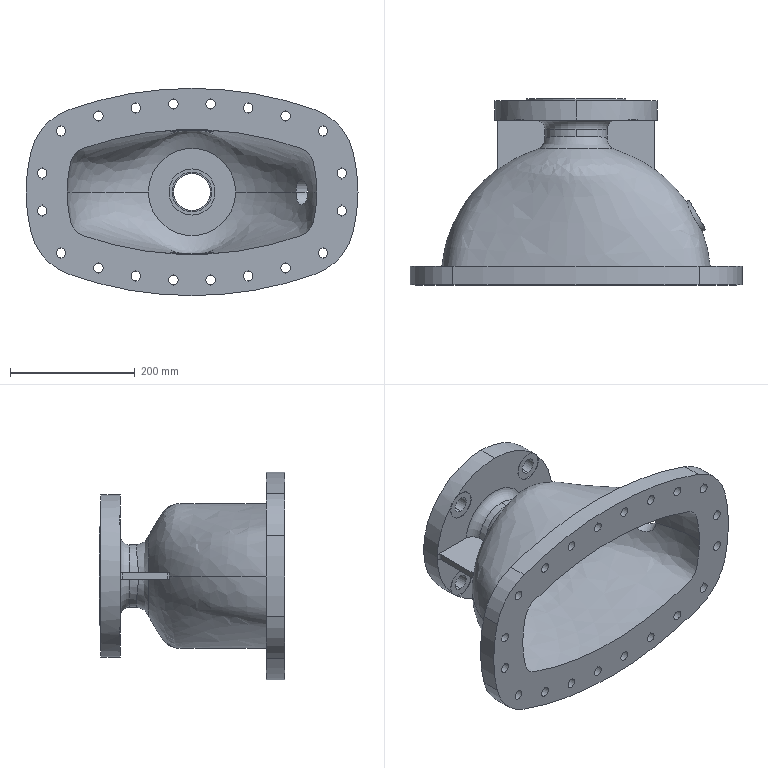Part | SolidWorks | features ICE 8, HoleWzd 4, Fillet 3, MirrorPattern 2, Blend 1, Chamfer 1, MoveFace 1, Revolution 1, Rib 1, Shell 1 | 1 solid | 239 faces | box 532 x 298 x 332 mm | volume 7097741 mm3 | cylinder 134 | cone 54 | plane 40 | spline 8 | torus 3 | commonest cylinder face diameters 22 x40 40 x40 46 x12 25 x8 14 x4 192 x4